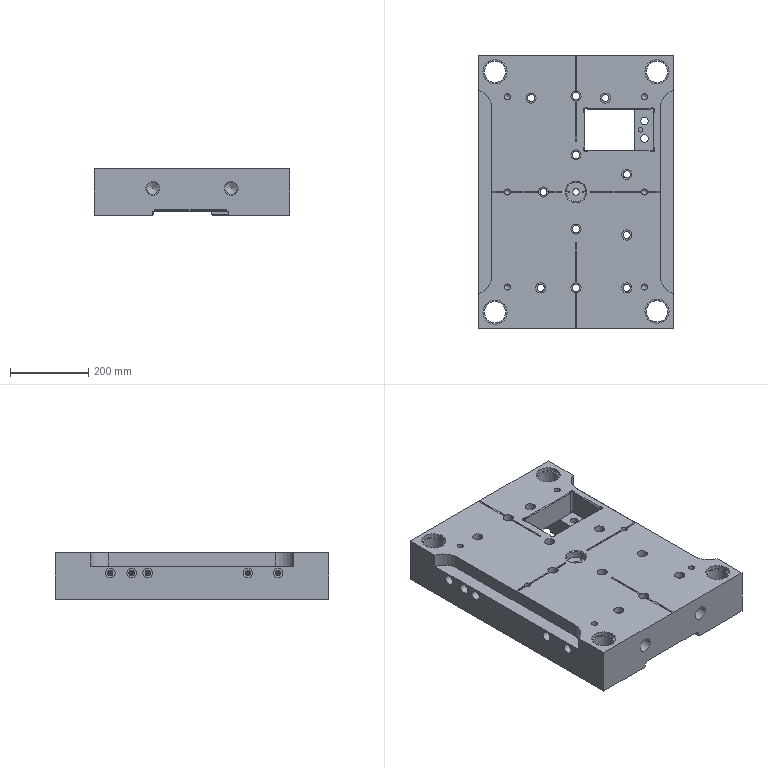Part | STEP file | AA | 1 solid | 568 faces | box 500 x 700 x 120 mm | volume 27100878 mm3 | plane 280 | cylinder 184 | cone 96 | spline 8 | commonest cylinder face diameters 10 x30 12 x30 16 x18 18 x11 26 x11 6.7 x8